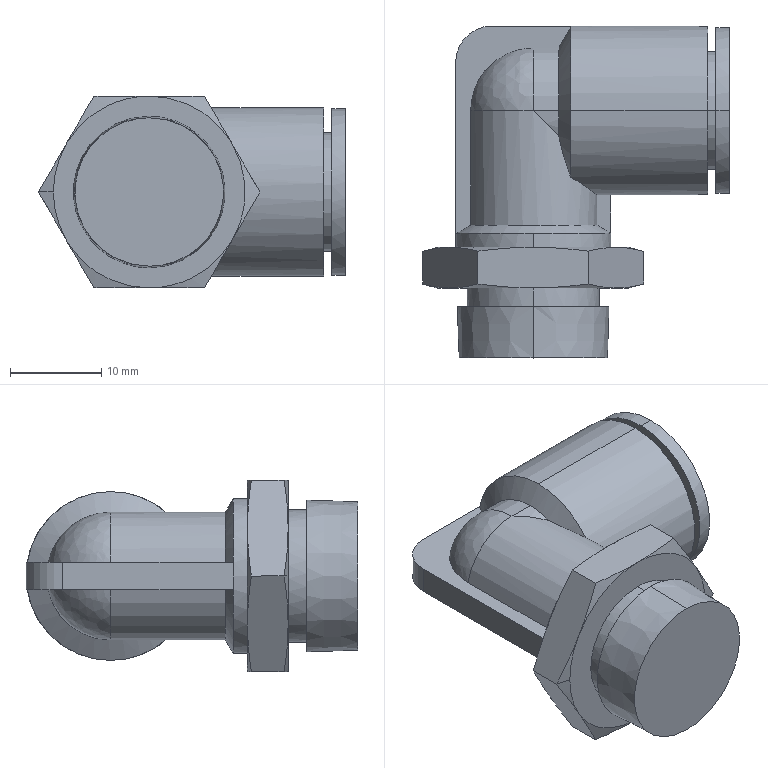Part | SolidWorks | features BaseBody 1 | 1 solid | 65 faces | box 33.624 x 36.35 x 21 mm | volume 9019 mm3 | plane 25 | cylinder 19 | cone 19 | spline 2 | commonest cylinder face diameters 14 x6 12 x2 12.95 x2 14.5 x2 17 x2 18.2 x2